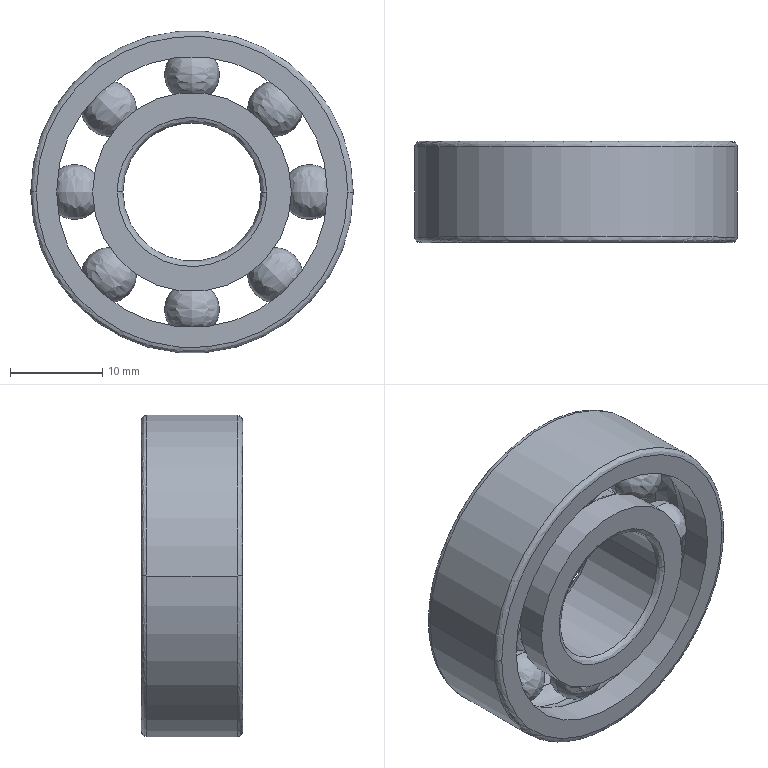Part | SolidWorks | features BaseBody 10 | 10 solids | 46 faces | box 35 x 11 x 35 mm | volume 5549 mm3 | spline 30 | cylinder 12 | plane 4 | commonest cylinder face diameters 21.6 x4 29.4 x4 15 x2 35 x2